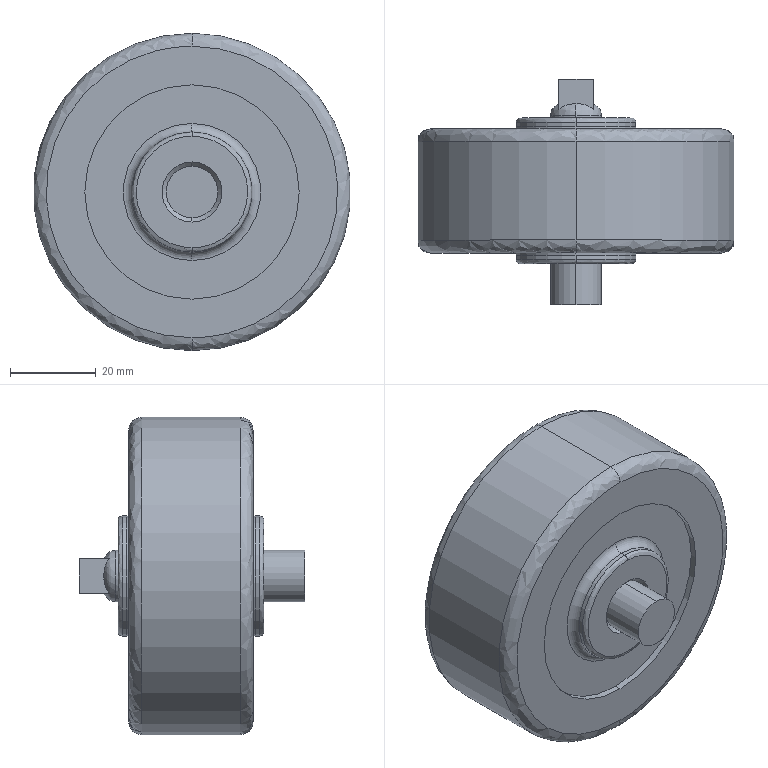Part | SolidWorks | features BaseBody 1 | 1 solid | 44 faces | box 74 x 52.5 x 74 mm | volume 124729 mm3 | cylinder 14 | plane 12 | spline 10 | torus 4 | cone 4 | commonest cylinder face diameters 12 x4 28 x4 50 x4 74 x2